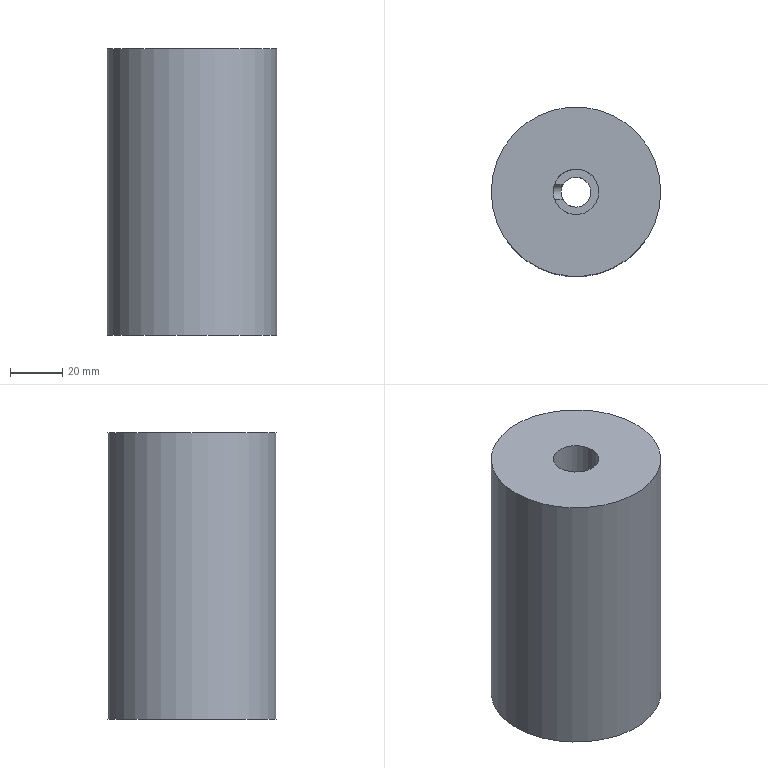Part | NX | features solid 2 | 1 solid | 8 faces | box 65 x 65 x 110 mm | volume 340839 mm3 | cylinder 4 | plane 4 | commonest cylinder face diameters 6 x1 11.5 x1 17.5 x1 65 x1
STEP:
#1=CARTESIAN_POINT('',(-893.22,347.,-35.));
#2=VERTEX_POINT('',#1);
#3=CARTESIAN_POINT('',(-893.22,353.,-35.));
#4=VERTEX_POINT('',#3);
#5=CARTESIAN_POINT('',(-893.22,347.,-35.));
#6=CARTESIAN_POINT('',(-893.22,347.,-34.201));
#7=CARTESIAN_POINT('',(-893.493,347.65,-32.657));
#8=CARTESIAN_POINT('',(-893.878,349.995,-31.672));
#9=CARTESIAN_POINT('',(-893.493,352.352,-32.656));
#10=CARTESIAN_POINT('',(-893.22,353.,-34.201));
#11=CARTESIAN_POINT('',(-893.22,353.,-35.));
#12=B_SPLINE_CURVE_WITH_KNOTS('',3,(#5,#6,#7,#8,#9,#10,#11),.UNSPECIFIED.,.F.,.F.,(4,1,1,1,4),(0.,0.002362,0.004724,0.007086,0.009448),.UNSPECIFIED.);
#13=EDGE_CURVE('',#2,#4,#12,.T.);
#14=ORIENTED_EDGE('',*,*,#13,.F.);
#15=CARTESIAN_POINT('',(-889.905,347.,-35.));
#16=VERTEX_POINT('',#15);
#17=CARTESIAN_POINT('',(-909.,347.,-35.));
#18=DIRECTION('',(1.,0.,0.));
#19=VECTOR('',#18,1000.);
#20=LINE('',#17,#19);
#21=EDGE_CURVE('',#16,#2,#20,.F.);
#22=ORIENTED_EDGE('',*,*,#21,.F.);
#23=CARTESIAN_POINT('',(-889.905,353.,-35.));
#24=VERTEX_POINT('',#23);
#25=CARTESIAN_POINT('',(-889.905,353.,-35.));
#26=CARTESIAN_POINT('',(-889.905,353.,-35.809));
#27=CARTESIAN_POINT('',(-890.359,352.352,-37.334));
#28=CARTESIAN_POINT('',(-890.945,350.008,-38.333));
#29=CARTESIAN_POINT('',(-890.36,347.645,-37.335));
#30=CARTESIAN_POINT('',(-889.905,347.,-35.81));
#31=CARTESIAN_POINT('',(-889.905,347.,-35.));
#32=B_SPLINE_CURVE_WITH_KNOTS('',3,(#25,#26,#27,#28,#29,#30,#31),.UNSPECIFIED.,.F.,.F.,(4,1,1,1,4),(0.,0.002388,0.004776,0.007165,0.009553),.UNSPECIFIED.);
#33=EDGE_CURVE('',#24,#16,#32,.T.);
#34=ORIENTED_EDGE('',*,*,#33,.F.);
#35=CARTESIAN_POINT('',(-909.,353.,-35.));
#36=DIRECTION('',(1.,0.,0.));
#37=VECTOR('',#36,1000.);
#38=LINE('',#35,#37);
#39=EDGE_CURVE('',#4,#24,#38,.T.);
#40=ORIENTED_EDGE('',*,*,#39,.F.);
#41=EDGE_LOOP('',(#14,#22,#34,#40));
#42=FACE_BOUND('',#41,.T.);
#43=CARTESIAN_POINT('',(-908.,350.,-32.));
#44=VERTEX_POINT('',#43);
#45=CARTESIAN_POINT('',(-908.,350.,-35.));
#46=DIRECTION('',(-1.,0.,0.));
#47=DIRECTION('',(0.,0.,1.));
#48=AXIS2_PLACEMENT_3D('',#45,#46,#47);
#49=CIRCLE('',#48,3.);
#50=EDGE_CURVE('',#44,#44,#49,.F.);
#51=ORIENTED_EDGE('',*,*,#50,.F.);
#52=EDGE_LOOP('',(#51));
#53=FACE_BOUND('',#52,.T.);
#54=CARTESIAN_POINT('',(-909.,350.,-35.));
#55=DIRECTION('',(1.,0.,0.));
#56=DIRECTION('',(0.,0.,1.));
#57=AXIS2_PLACEMENT_3D('',#54,#55,#56);
#58=CYLINDRICAL_SURFACE('',#57,3.);
#59=ADVANCED_FACE('',(#42,#53),#58,.F.);
#60=CARTESIAN_POINT('',(-876.25,350.,55.));
#61=VERTEX_POINT('',#60);
#62=CARTESIAN_POINT('',(-885.,350.,55.));
#63=DIRECTION('',(0.,0.,-1.));
#64=DIRECTION('',(1.,0.,0.));
#65=AXIS2_PLACEMENT_3D('',#62,#63,#64);
#66=CIRCLE('',#65,8.75);
#67=EDGE_CURVE('',#61,#61,#66,.T.);
#68=ORIENTED_EDGE('',*,*,#67,.T.);
#69=EDGE_LOOP('',(#68));
#70=FACE_BOUND('',#69,.T.);
#71=CARTESIAN_POINT('',(-852.5,350.,55.));
#72=VERTEX_POINT('',#71);
#73=CARTESIAN_POINT('',(-885.,350.,55.));
#74=DIRECTION('',(0.,0.,-1.));
#75=DIRECTION('',(1.,0.,0.));
#76=AXIS2_PLACEMENT_3D('',#73,#74,#75);
#77=CIRCLE('',#76,32.5);
#78=EDGE_CURVE('',#72,#72,#77,.T.);
#79=ORIENTED_EDGE('',*,*,#78,.F.);
#80=EDGE_LOOP('',(#79));
#81=FACE_BOUND('',#80,.T.);
#82=CARTESIAN_POINT('',(-885.,350.,55.));
#83=DIRECTION('',(0.,0.,1.));
#84=DIRECTION('',(-1.,0.,0.));
#85=AXIS2_PLACEMENT_3D('',#82,#83,#84);
#86=PLANE('',#85);
#87=ADVANCED_FACE('',(#70,#81),#86,.T.);
#88=CARTESIAN_POINT('',(-852.5,350.,-55.));
#89=VERTEX_POINT('',#88);
#90=CARTESIAN_POINT('',(-885.,350.,-55.));
#91=DIRECTION('',(0.,0.,-1.));
#92=DIRECTION('',(1.,0.,0.));
#93=AXIS2_PLACEMENT_3D('',#90,#91,#92);
#94=CIRCLE('',#93,32.5);
#95=EDGE_CURVE('',#89,#89,#94,.T.);
#96=ORIENTED_EDGE('',*,*,#95,.T.);
#97=EDGE_LOOP('',(#96));
#98=FACE_BOUND('',#97,.T.);
#99=CARTESIAN_POINT('',(-890.75,350.,-55.));
#100=VERTEX_POINT('',#99);
#101=CARTESIAN_POINT('',(-885.,350.,-55.));
#102=DIRECTION('',(0.,0.,-1.));
#103=DIRECTION('',(-1.,0.,0.));
#104=AXIS2_PLACEMENT_3D('',#101,#102,#103);
#105=CIRCLE('',#104,5.75);
#106=EDGE_CURVE('',#100,#100,#105,.T.);
#107=ORIENTED_EDGE('',*,*,#106,.F.);
#108=EDGE_LOOP('',(#107));
#109=FACE_BOUND('',#108,.T.);
#110=CARTESIAN_POINT('',(-885.,350.,-55.));
#111=DIRECTION('',(0.,0.,1.));
#112=DIRECTION('',(-1.,0.,0.));
#113=AXIS2_PLACEMENT_3D('',#110,#111,#112);
#114=PLANE('',#113);
#115=ADVANCED_FACE('',(#98,#109),#114,.F.);
#116=ORIENTED_EDGE('',*,*,#39,.T.);
#117=CARTESIAN_POINT('',(-885.,350.,-35.));
#118=DIRECTION('',(0.,0.,-1.));
#119=DIRECTION('',(-1.,0.,0.));
#120=AXIS2_PLACEMENT_3D('',#117,#118,#119);
#121=CIRCLE('',#120,5.75);
#122=EDGE_CURVE('',#24,#16,#121,.T.);
#123=ORIENTED_EDGE('',*,*,#122,.T.);
#124=ORIENTED_EDGE('',*,*,#21,.T.);
#125=CARTESIAN_POINT('',(-885.,350.,-35.));
#126=DIRECTION('',(0.,0.,-1.));
#127=DIRECTION('',(-1.,0.,0.));
#128=AXIS2_PLACEMENT_3D('',#125,#126,#127);
#129=CIRCLE('',#128,8.75);
#130=EDGE_CURVE('',#4,#2,#129,.T.);
#131=ORIENTED_EDGE('',*,*,#130,.F.);
#132=EDGE_LOOP('',(#116,#123,#124,#131));
#133=FACE_BOUND('',#132,.T.);
#134=CARTESIAN_POINT('',(-885.,350.,-35.));
#135=DIRECTION('',(0.,0.,1.));
#136=DIRECTION('',(-1.,0.,0.));
#137=AXIS2_PLACEMENT_3D('',#134,#135,#136);
#138=PLANE('',#137);
#139=ADVANCED_FACE('',(#133),#138,.T.);
#140=ORIENTED_EDGE('',*,*,#78,.T.);
#141=EDGE_LOOP('',(#140));
#142=FACE_BOUND('',#141,.T.);
#143=ORIENTED_EDGE('',*,*,#95,.F.);
#144=EDGE_LOOP('',(#143));
#145=FACE_BOUND('',#144,.T.);
#146=CARTESIAN_POINT('',(-885.,350.,-15.));
#147=DIRECTION('',(0.,0.,-1.));
#148=DIRECTION('',(1.,0.,0.));
#149=AXIS2_PLACEMENT_3D('',#146,#147,#148);
#150=CYLINDRICAL_SURFACE('',#149,32.5);
#151=ADVANCED_FACE('',(#142,#145),#150,.T.);
#152=ORIENTED_EDGE('',*,*,#13,.T.);
#153=ORIENTED_EDGE('',*,*,#130,.T.);
#154=EDGE_LOOP('',(#152,#153));
#155=FACE_BOUND('',#154,.T.);
#156=ORIENTED_EDGE('',*,*,#67,.F.);
#157=EDGE_LOOP('',(#156));
#158=FACE_BOUND('',#157,.T.);
#159=CARTESIAN_POINT('',(-885.,350.,-15.));
#160=DIRECTION('',(0.,0.,-1.));
#161=DIRECTION('',(1.,0.,0.));
#162=AXIS2_PLACEMENT_3D('',#159,#160,#161);
#163=CYLINDRICAL_SURFACE('',#162,8.75);
#164=ADVANCED_FACE('',(#155,#158),#163,.F.);
#165=ORIENTED_EDGE('',*,*,#33,.T.);
#166=ORIENTED_EDGE('',*,*,#122,.F.);
#167=EDGE_LOOP('',(#165,#166));
#168=FACE_BOUND('',#167,.T.);
#169=ORIENTED_EDGE('',*,*,#106,.T.);
#170=EDGE_LOOP('',(#169));
#171=FACE_BOUND('',#170,.T.);
#172=CARTESIAN_POINT('',(-885.,350.,-35.));
#173=DIRECTION('',(0.,0.,-1.));
#174=DIRECTION('',(1.,0.,0.));
#175=AXIS2_PLACEMENT_3D('',#172,#173,#174);
#176=CYLINDRICAL_SURFACE('',#175,5.75);
#177=ADVANCED_FACE('',(#168,#171),#176,.F.);
#178=ORIENTED_EDGE('',*,*,#50,.T.);
#179=EDGE_LOOP('',(#178));
#180=FACE_BOUND('',#179,.T.);
#181=CARTESIAN_POINT('',(-908.,350.,-35.));
#182=DIRECTION('',(-1.,0.,0.));
#183=DIRECTION('',(0.,0.,1.));
#184=AXIS2_PLACEMENT_3D('',#181,#182,#183);
#185=PLANE('',#184);
#186=ADVANCED_FACE('',(#180),#185,.F.);
#187=CLOSED_SHELL('',(#59,#87,#115,#139,#151,#164,#177,#186));
#188=MANIFOLD_SOLID_BREP('',#187);
#189=(LENGTH_UNIT()NAMED_UNIT(*)SI_UNIT(.MILLI.,.METRE.));
#190=UNCERTAINTY_MEASURE_WITH_UNIT(LENGTH_MEASURE(0.0508),#189,'','');
#191=(NAMED_UNIT(*)PLANE_ANGLE_UNIT()SI_UNIT($,.RADIAN.));
#192=(NAMED_UNIT(*)SI_UNIT($,.STERADIAN.)SOLID_ANGLE_UNIT());
#193=(GEOMETRIC_REPRESENTATION_CONTEXT(3)GLOBAL_UNCERTAINTY_ASSIGNED_CONTEXT((#190))GLOBAL_UNIT_ASSIGNED_CONTEXT((#189,#191,#192))REPRESENTATION_CONTEXT('',''));
#194=ADVANCED_BREP_SHAPE_REPRESENTATION('',(#188),#193);